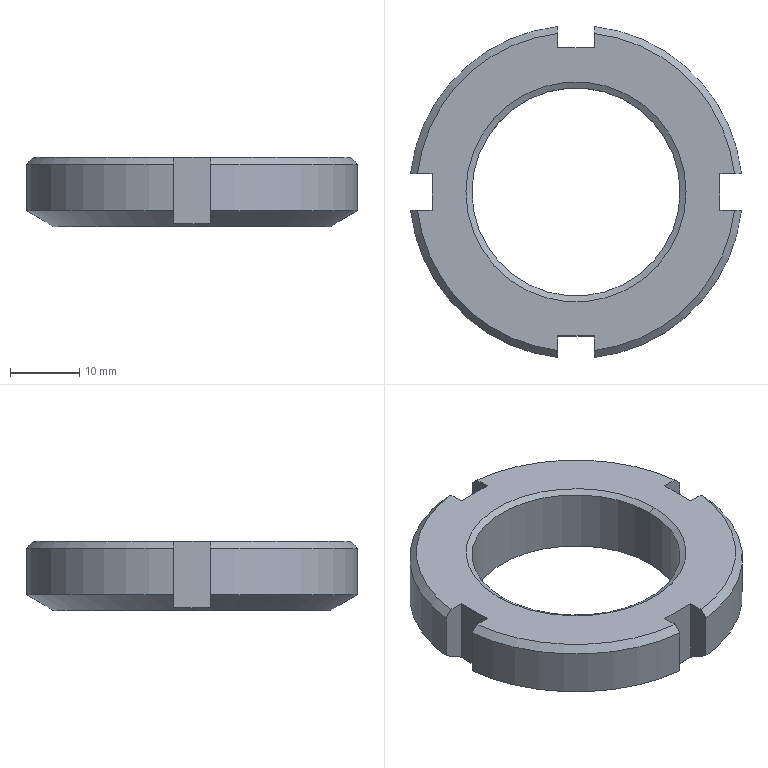Part | SolidWorks | features Chamfer 3, CirPattern 1, Cut 1, Extrusion 1 | 1 solid | 30 faces | box 47.706 x 47.706 x 10 mm | volume 9680 mm3 | plane 14 | cone 10 | cylinder 6 | commonest cylinder face diameters 48 x4 30 x2
STEP:
#1=CARTESIAN_POINT('',(-15.,0.,9.5));
#2=VERTEX_POINT('',#1);
#3=CARTESIAN_POINT('',(15.,0.,9.5));
#4=VERTEX_POINT('',#3);
#5=CARTESIAN_POINT('',(0.,0.,9.5));
#6=DIRECTION('',(0.,0.,1.));
#7=DIRECTION('',(1.,0.,0.));
#8=AXIS2_PLACEMENT_3D('',#5,#6,#7);
#9=CIRCLE('',#8,15.);
#10=EDGE_CURVE('',#2,#4,#9,.T.);
#11=ORIENTED_EDGE('',*,*,#10,.F.);
#12=CARTESIAN_POINT('',(-15.866,0.,10.));
#13=VERTEX_POINT('',#12);
#14=CARTESIAN_POINT('',(-15.,0.,9.5));
#15=DIRECTION('',(-0.866,0.,0.5));
#16=VECTOR('',#15,1000.);
#17=LINE('',#14,#16);
#18=EDGE_CURVE('',#2,#13,#17,.T.);
#19=ORIENTED_EDGE('',*,*,#18,.T.);
#20=CARTESIAN_POINT('',(15.866,0.,10.));
#21=VERTEX_POINT('',#20);
#22=CARTESIAN_POINT('',(0.,0.,10.));
#23=DIRECTION('',(0.,0.,-1.));
#24=DIRECTION('',(1.,0.,0.));
#25=AXIS2_PLACEMENT_3D('',#22,#23,#24);
#26=CIRCLE('',#25,15.866);
#27=EDGE_CURVE('',#21,#13,#26,.T.);
#28=ORIENTED_EDGE('',*,*,#27,.F.);
#29=CARTESIAN_POINT('',(15.,0.,9.5));
#30=DIRECTION('',(0.866,0.,0.5));
#31=VECTOR('',#30,1000.);
#32=LINE('',#29,#31);
#33=EDGE_CURVE('',#4,#21,#32,.T.);
#34=ORIENTED_EDGE('',*,*,#33,.F.);
#35=EDGE_LOOP('',(#11,#19,#28,#34));
#36=FACE_OUTER_BOUND('',#35,.T.);
#37=CARTESIAN_POINT('',(0.,0.,9.5));
#38=DIRECTION('',(0.,0.,1.));
#39=DIRECTION('',(1.,0.,0.));
#40=AXIS2_PLACEMENT_3D('',#37,#38,#39);
#41=CONICAL_SURFACE('',#40,15.,1.047);
#42=ADVANCED_FACE('',(#36),#41,.F.);
#43=CARTESIAN_POINT('',(15.,0.,0.5));
#44=VERTEX_POINT('',#43);
#45=CARTESIAN_POINT('',(-15.,0.,0.5));
#46=VERTEX_POINT('',#45);
#47=CARTESIAN_POINT('',(0.,0.,0.5));
#48=DIRECTION('',(0.,0.,-1.));
#49=DIRECTION('',(1.,0.,0.));
#50=AXIS2_PLACEMENT_3D('',#47,#48,#49);
#51=CIRCLE('',#50,15.);
#52=EDGE_CURVE('',#44,#46,#51,.T.);
#53=ORIENTED_EDGE('',*,*,#52,.F.);
#54=CARTESIAN_POINT('',(15.866,0.,0.));
#55=VERTEX_POINT('',#54);
#56=CARTESIAN_POINT('',(15.866,0.,0.));
#57=DIRECTION('',(0.866,0.,-0.5));
#58=VECTOR('',#57,1000.);
#59=LINE('',#56,#58);
#60=EDGE_CURVE('',#44,#55,#59,.T.);
#61=ORIENTED_EDGE('',*,*,#60,.T.);
#62=CARTESIAN_POINT('',(-15.866,0.,0.));
#63=VERTEX_POINT('',#62);
#64=CARTESIAN_POINT('',(0.,0.,0.));
#65=DIRECTION('',(0.,0.,1.));
#66=DIRECTION('',(1.,0.,0.));
#67=AXIS2_PLACEMENT_3D('',#64,#65,#66);
#68=CIRCLE('',#67,15.866);
#69=EDGE_CURVE('',#63,#55,#68,.T.);
#70=ORIENTED_EDGE('',*,*,#69,.F.);
#71=CARTESIAN_POINT('',(-15.866,0.,0.));
#72=DIRECTION('',(-0.866,0.,-0.5));
#73=VECTOR('',#72,1000.);
#74=LINE('',#71,#73);
#75=EDGE_CURVE('',#46,#63,#74,.T.);
#76=ORIENTED_EDGE('',*,*,#75,.F.);
#77=EDGE_LOOP('',(#53,#61,#70,#76));
#78=FACE_OUTER_BOUND('',#77,.T.);
#79=CARTESIAN_POINT('',(0.,0.,0.));
#80=DIRECTION('',(0.,0.,-1.));
#81=DIRECTION('',(-1.,0.,0.));
#82=AXIS2_PLACEMENT_3D('',#79,#80,#81);
#83=CONICAL_SURFACE('',#82,15.866,1.047);
#84=ADVANCED_FACE('',(#78),#83,.F.);
#85=CARTESIAN_POINT('',(-20.,0.,0.));
#86=VERTEX_POINT('',#85);
#87=CARTESIAN_POINT('',(20.,0.,0.));
#88=VERTEX_POINT('',#87);
#89=CARTESIAN_POINT('',(0.,0.,0.));
#90=DIRECTION('',(0.,0.,-1.));
#91=DIRECTION('',(1.,0.,0.));
#92=AXIS2_PLACEMENT_3D('',#89,#90,#91);
#93=CIRCLE('',#92,20.);
#94=EDGE_CURVE('',#86,#88,#93,.T.);
#95=ORIENTED_EDGE('',*,*,#94,.F.);
#96=CARTESIAN_POINT('',(-20.753,0.,0.4349));
#97=VERTEX_POINT('',#96);
#98=CARTESIAN_POINT('',(-24.,0.,2.309));
#99=DIRECTION('',(-0.866,0.,0.5));
#100=VECTOR('',#99,1000.);
#101=LINE('',#98,#100);
#102=EDGE_CURVE('',#86,#97,#101,.T.);
#103=ORIENTED_EDGE('',*,*,#102,.T.);
#104=CARTESIAN_POINT('',(-20.753,2.65,0.5322));
#105=VERTEX_POINT('',#104);
#106=CARTESIAN_POINT('',(-20.753,2.65,0.5322));
#107=CARTESIAN_POINT('',(-20.753,1.77,0.4678));
#108=CARTESIAN_POINT('',(-20.753,0.8866,0.4349));
#109=CARTESIAN_POINT('',(-20.753,0.,0.4349));
#110=B_SPLINE_CURVE_WITH_KNOTS('',3,(#106,#107,#108,#109),.UNSPECIFIED.,.F.,.F.,(4,4),(0.007091,0.009737),.UNSPECIFIED.);
#111=EDGE_CURVE('',#105,#97,#110,.T.);
#112=ORIENTED_EDGE('',*,*,#111,.F.);
#113=CARTESIAN_POINT('',(-23.853,2.65,2.309));
#114=VERTEX_POINT('',#113);
#115=CARTESIAN_POINT('',(-23.853,2.65,2.309));
#116=CARTESIAN_POINT('',(-22.82,2.65,1.717));
#117=CARTESIAN_POINT('',(-21.787,2.65,1.124));
#118=CARTESIAN_POINT('',(-20.753,2.65,0.5322));
#119=B_SPLINE_CURVE_WITH_KNOTS('',3,(#115,#116,#117,#118),.UNSPECIFIED.,.F.,.F.,(4,4),(0.00673,0.0103),.UNSPECIFIED.);
#120=EDGE_CURVE('',#114,#105,#119,.T.);
#121=ORIENTED_EDGE('',*,*,#120,.F.);
#122=CARTESIAN_POINT('',(-2.65,23.853,2.309));
#123=VERTEX_POINT('',#122);
#124=CARTESIAN_POINT('',(0.,0.,2.309));
#125=DIRECTION('',(0.,0.,1.));
#126=DIRECTION('',(1.,0.,0.));
#127=AXIS2_PLACEMENT_3D('',#124,#125,#126);
#128=CIRCLE('',#127,24.);
#129=EDGE_CURVE('',#123,#114,#128,.T.);
#130=ORIENTED_EDGE('',*,*,#129,.F.);
#131=CARTESIAN_POINT('',(-2.65,20.753,0.5322));
#132=VERTEX_POINT('',#131);
#133=CARTESIAN_POINT('',(-2.65,20.753,0.5322));
#134=CARTESIAN_POINT('',(-2.65,21.787,1.124));
#135=CARTESIAN_POINT('',(-2.65,22.82,1.717));
#136=CARTESIAN_POINT('',(-2.65,23.853,2.309));
#137=B_SPLINE_CURVE_WITH_KNOTS('',3,(#133,#134,#135,#136),.UNSPECIFIED.,.F.,.F.,(4,4),(0.006995,0.01057),.UNSPECIFIED.);
#138=EDGE_CURVE('',#132,#123,#137,.T.);
#139=ORIENTED_EDGE('',*,*,#138,.F.);
#140=CARTESIAN_POINT('',(2.65,20.753,0.5322));
#141=VERTEX_POINT('',#140);
#142=CARTESIAN_POINT('',(2.65,20.753,0.5322));
#143=CARTESIAN_POINT('',(1.773,20.753,0.468));
#144=CARTESIAN_POINT('',(0.8926,20.753,0.4351));
#145=CARTESIAN_POINT('',(-0.8746,20.753,0.4347));
#146=CARTESIAN_POINT('',(-1.764,20.753,0.4674));
#147=CARTESIAN_POINT('',(-2.65,20.753,0.5322));
#148=B_SPLINE_CURVE_WITH_KNOTS('',3,(#142,#143,#144,#145,#146,#147),.UNSPECIFIED.,.F.,.F.,(4,2,4),(0.007091,0.009729,0.01237),.UNSPECIFIED.);
#149=EDGE_CURVE('',#141,#132,#148,.T.);
#150=ORIENTED_EDGE('',*,*,#149,.F.);
#151=CARTESIAN_POINT('',(2.65,23.853,2.309));
#152=VERTEX_POINT('',#151);
#153=CARTESIAN_POINT('',(2.65,23.853,2.309));
#154=CARTESIAN_POINT('',(2.65,22.82,1.717));
#155=CARTESIAN_POINT('',(2.65,21.787,1.124));
#156=CARTESIAN_POINT('',(2.65,20.753,0.5322));
#157=B_SPLINE_CURVE_WITH_KNOTS('',3,(#153,#154,#155,#156),.UNSPECIFIED.,.F.,.F.,(4,4),(0.004139,0.007712),.UNSPECIFIED.);
#158=EDGE_CURVE('',#152,#141,#157,.T.);
#159=ORIENTED_EDGE('',*,*,#158,.F.);
#160=CARTESIAN_POINT('',(23.853,2.65,2.309));
#161=VERTEX_POINT('',#160);
#162=CARTESIAN_POINT('',(0.,0.,2.309));
#163=DIRECTION('',(0.,0.,1.));
#164=DIRECTION('',(1.,0.,0.));
#165=AXIS2_PLACEMENT_3D('',#162,#163,#164);
#166=CIRCLE('',#165,24.);
#167=EDGE_CURVE('',#161,#152,#166,.T.);
#168=ORIENTED_EDGE('',*,*,#167,.F.);
#169=CARTESIAN_POINT('',(20.753,2.65,0.5322));
#170=VERTEX_POINT('',#169);
#171=CARTESIAN_POINT('',(20.753,2.65,0.5322));
#172=CARTESIAN_POINT('',(21.787,2.65,1.124));
#173=CARTESIAN_POINT('',(22.82,2.65,1.717));
#174=CARTESIAN_POINT('',(23.853,2.65,2.309));
#175=B_SPLINE_CURVE_WITH_KNOTS('',3,(#171,#172,#173,#174),.UNSPECIFIED.,.F.,.F.,(4,4),(0.006995,0.01057),.UNSPECIFIED.);
#176=EDGE_CURVE('',#170,#161,#175,.T.);
#177=ORIENTED_EDGE('',*,*,#176,.F.);
#178=CARTESIAN_POINT('',(20.753,0.,0.4349));
#179=VERTEX_POINT('',#178);
#180=CARTESIAN_POINT('',(20.753,0.,0.4349));
#181=CARTESIAN_POINT('',(20.753,0.8866,0.4349));
#182=CARTESIAN_POINT('',(20.753,1.77,0.4678));
#183=CARTESIAN_POINT('',(20.753,2.65,0.5322));
#184=B_SPLINE_CURVE_WITH_KNOTS('',3,(#180,#181,#182,#183),.UNSPECIFIED.,.F.,.F.,(4,4),(0.01366,0.01632),.UNSPECIFIED.);
#185=EDGE_CURVE('',#179,#170,#184,.T.);
#186=ORIENTED_EDGE('',*,*,#185,.F.);
#187=CARTESIAN_POINT('',(24.,0.,2.309));
#188=DIRECTION('',(0.866,0.,0.5));
#189=VECTOR('',#188,1000.);
#190=LINE('',#187,#189);
#191=EDGE_CURVE('',#88,#179,#190,.T.);
#192=ORIENTED_EDGE('',*,*,#191,.F.);
#193=EDGE_LOOP('',(#95,#103,#112,#121,#130,#139,#150,#159,#168,#177,#186,#192));
#194=FACE_OUTER_BOUND('',#193,.T.);
#195=CARTESIAN_POINT('',(0.,0.,2.309));
#196=DIRECTION('',(0.,0.,1.));
#197=DIRECTION('',(1.,0.,0.));
#198=AXIS2_PLACEMENT_3D('',#195,#196,#197);
#199=CONICAL_SURFACE('',#198,24.,1.047);
#200=ADVANCED_FACE('',(#194),#199,.T.);
#201=ORIENTED_EDGE('',*,*,#10,.T.);
#202=CARTESIAN_POINT('',(15.,0.,10.));
#203=DIRECTION('',(0.,0.,-1.));
#204=VECTOR('',#203,1000.);
#205=LINE('',#202,#204);
#206=EDGE_CURVE('',#4,#44,#205,.T.);
#207=ORIENTED_EDGE('',*,*,#206,.T.);
#208=ORIENTED_EDGE('',*,*,#52,.T.);
#209=CARTESIAN_POINT('',(-15.,0.,10.));
#210=DIRECTION('',(0.,0.,-1.));
#211=VECTOR('',#210,1000.);
#212=LINE('',#209,#211);
#213=EDGE_CURVE('',#2,#46,#212,.T.);
#214=ORIENTED_EDGE('',*,*,#213,.F.);
#215=EDGE_LOOP('',(#201,#207,#208,#214));
#216=FACE_OUTER_BOUND('',#215,.T.);
#217=CARTESIAN_POINT('',(0.,0.,10.));
#218=DIRECTION('',(0.,0.,-1.));
#219=DIRECTION('',(-1.,0.,0.));
#220=AXIS2_PLACEMENT_3D('',#217,#218,#219);
#221=CYLINDRICAL_SURFACE('',#220,15.);
#222=ADVANCED_FACE('',(#216),#221,.F.);
#223=CARTESIAN_POINT('',(2.65,23.853,9.));
#224=VERTEX_POINT('',#223);
#225=CARTESIAN_POINT('',(23.853,2.65,9.));
#226=VERTEX_POINT('',#225);
#227=CARTESIAN_POINT('',(0.,0.,9.));
#228=DIRECTION('',(0.,0.,-1.));
#229=DIRECTION('',(1.,0.,0.));
#230=AXIS2_PLACEMENT_3D('',#227,#228,#229);
#231=CIRCLE('',#230,24.);
#232=EDGE_CURVE('',#224,#226,#231,.T.);
#233=ORIENTED_EDGE('',*,*,#232,.T.);
#234=CARTESIAN_POINT('',(23.853,2.65,0.));
#235=DIRECTION('',(0.,0.,1.));
#236=VECTOR('',#235,1000.);
#237=LINE('',#234,#236);
#238=EDGE_CURVE('',#161,#226,#237,.T.);
#239=ORIENTED_EDGE('',*,*,#238,.F.);
#240=ORIENTED_EDGE('',*,*,#167,.T.);
#241=CARTESIAN_POINT('',(2.65,23.853,0.));
#242=DIRECTION('',(0.,0.,1.));
#243=VECTOR('',#242,1000.);
#244=LINE('',#241,#243);
#245=EDGE_CURVE('',#152,#224,#244,.T.);
#246=ORIENTED_EDGE('',*,*,#245,.T.);
#247=EDGE_LOOP('',(#233,#239,#240,#246));
#248=FACE_OUTER_BOUND('',#247,.T.);
#249=CARTESIAN_POINT('',(0.,0.,10.));
#250=DIRECTION('',(0.,0.,-1.));
#251=DIRECTION('',(-1.,0.,0.));
#252=AXIS2_PLACEMENT_3D('',#249,#250,#251);
#253=CYLINDRICAL_SURFACE('',#252,24.);
#254=ADVANCED_FACE('',(#248),#253,.T.);
#255=CARTESIAN_POINT('',(22.847,2.65,10.));
#256=VERTEX_POINT('',#255);
#257=CARTESIAN_POINT('',(23.853,2.65,9.));
#258=CARTESIAN_POINT('',(23.575,2.65,9.277));
#259=CARTESIAN_POINT('',(23.297,2.65,9.553));
#260=CARTESIAN_POINT('',(23.018,2.65,9.83));
#261=CARTESIAN_POINT('',(22.961,2.65,9.886));
#262=CARTESIAN_POINT('',(22.904,2.65,9.943));
#263=CARTESIAN_POINT('',(22.847,2.65,10.));
#264=B_SPLINE_CURVE_WITH_KNOTS('',3,(#257,#258,#259,#260,#261,#262,#263),.UNSPECIFIED.,.F.,.F.,(4,3,4),(0.005158,0.006335,0.006577),.UNSPECIFIED.);
#265=EDGE_CURVE('',#226,#256,#264,.T.);
#266=ORIENTED_EDGE('',*,*,#265,.F.);
#267=ORIENTED_EDGE('',*,*,#232,.F.);
#268=CARTESIAN_POINT('',(2.65,22.847,10.));
#269=VERTEX_POINT('',#268);
#270=CARTESIAN_POINT('',(2.65,22.847,10.));
#271=CARTESIAN_POINT('',(2.65,22.904,9.943));
#272=CARTESIAN_POINT('',(2.65,22.961,9.886));
#273=CARTESIAN_POINT('',(2.65,23.018,9.83));
#274=CARTESIAN_POINT('',(2.65,23.297,9.553));
#275=CARTESIAN_POINT('',(2.65,23.575,9.277));
#276=CARTESIAN_POINT('',(2.65,23.853,9.));
#277=B_SPLINE_CURVE_WITH_KNOTS('',3,(#270,#271,#272,#273,#274,#275,#276),.UNSPECIFIED.,.F.,.F.,(4,3,4),(0.006094,0.006335,0.007512),.UNSPECIFIED.);
#278=EDGE_CURVE('',#269,#224,#277,.T.);
#279=ORIENTED_EDGE('',*,*,#278,.F.);
#280=CARTESIAN_POINT('',(0.,0.,10.));
#281=DIRECTION('',(0.,0.,1.));
#282=DIRECTION('',(1.,0.,0.));
#283=AXIS2_PLACEMENT_3D('',#280,#281,#282);
#284=CIRCLE('',#283,23.);
#285=EDGE_CURVE('',#256,#269,#284,.T.);
#286=ORIENTED_EDGE('',*,*,#285,.F.);
#287=EDGE_LOOP('',(#266,#267,#279,#286));
#288=FACE_OUTER_BOUND('',#287,.T.);
#289=CARTESIAN_POINT('',(0.,0.,10.));
#290=DIRECTION('',(0.,0.,-1.));
#291=DIRECTION('',(-1.,0.,0.));
#292=AXIS2_PLACEMENT_3D('',#289,#290,#291);
#293=CONICAL_SURFACE('',#292,23.,0.7854);
#294=ADVANCED_FACE('',(#288),#293,.T.);
#295=CARTESIAN_POINT('',(-23.853,2.65,9.));
#296=VERTEX_POINT('',#295);
#297=CARTESIAN_POINT('',(-2.65,23.853,9.));
#298=VERTEX_POINT('',#297);
#299=CARTESIAN_POINT('',(0.,0.,9.));
#300=DIRECTION('',(0.,0.,-1.));
#301=DIRECTION('',(1.,0.,0.));
#302=AXIS2_PLACEMENT_3D('',#299,#300,#301);
#303=CIRCLE('',#302,24.);
#304=EDGE_CURVE('',#296,#298,#303,.T.);
#305=ORIENTED_EDGE('',*,*,#304,.T.);
#306=CARTESIAN_POINT('',(-2.65,23.853,0.));
#307=DIRECTION('',(0.,0.,1.));
#308=VECTOR('',#307,1000.);
#309=LINE('',#306,#308);
#310=EDGE_CURVE('',#123,#298,#309,.T.);
#311=ORIENTED_EDGE('',*,*,#310,.F.);
#312=ORIENTED_EDGE('',*,*,#129,.T.);
#313=CARTESIAN_POINT('',(-23.853,2.65,0.));
#314=DIRECTION('',(0.,0.,1.));
#315=VECTOR('',#314,1000.);
#316=LINE('',#313,#315);
#317=EDGE_CURVE('',#114,#296,#316,.T.);
#318=ORIENTED_EDGE('',*,*,#317,.T.);
#319=EDGE_LOOP('',(#305,#311,#312,#318));
#320=FACE_OUTER_BOUND('',#319,.T.);
#321=CARTESIAN_POINT('',(0.,0.,10.));
#322=DIRECTION('',(0.,0.,-1.));
#323=DIRECTION('',(-1.,0.,0.));
#324=AXIS2_PLACEMENT_3D('',#321,#322,#323);
#325=CYLINDRICAL_SURFACE('',#324,24.);
#326=ADVANCED_FACE('',(#320),#325,.T.);
#327=CARTESIAN_POINT('',(-2.65,22.847,10.));
#328=VERTEX_POINT('',#327);
#329=CARTESIAN_POINT('',(-2.65,23.853,9.));
#330=CARTESIAN_POINT('',(-2.65,23.575,9.277));
#331=CARTESIAN_POINT('',(-2.65,23.297,9.553));
#332=CARTESIAN_POINT('',(-2.65,23.018,9.83));
#333=CARTESIAN_POINT('',(-2.65,22.961,9.886));
#334=CARTESIAN_POINT('',(-2.65,22.904,9.943));
#335=CARTESIAN_POINT('',(-2.65,22.847,10.));
#336=B_SPLINE_CURVE_WITH_KNOTS('',3,(#329,#330,#331,#332,#333,#334,#335),.UNSPECIFIED.,.F.,.F.,(4,3,4),(0.005158,0.006335,0.006577),.UNSPECIFIED.);
#337=EDGE_CURVE('',#298,#328,#336,.T.);
#338=ORIENTED_EDGE('',*,*,#337,.F.);
#339=ORIENTED_EDGE('',*,*,#304,.F.);
#340=CARTESIAN_POINT('',(-22.847,2.65,10.));
#341=VERTEX_POINT('',#340);
#342=CARTESIAN_POINT('',(-22.847,2.65,10.));
#343=CARTESIAN_POINT('',(-23.034,2.65,9.814));
#344=CARTESIAN_POINT('',(-23.221,2.65,9.628));
#345=CARTESIAN_POINT('',(-23.408,2.65,9.442));
#346=CARTESIAN_POINT('',(-23.557,2.65,9.295));
#347=CARTESIAN_POINT('',(-23.705,2.65,9.147));
#348=CARTESIAN_POINT('',(-23.853,2.65,9.));
#349=B_SPLINE_CURVE_WITH_KNOTS('',3,(#342,#343,#344,#345,#346,#347,#348),.UNSPECIFIED.,.F.,.F.,(4,3,4),(0.005544,0.006335,0.006963),.UNSPECIFIED.);
#350=EDGE_CURVE('',#341,#296,#349,.T.);
#351=ORIENTED_EDGE('',*,*,#350,.F.);
#352=CARTESIAN_POINT('',(0.,0.,10.));
#353=DIRECTION('',(0.,0.,1.));
#354=DIRECTION('',(1.,0.,0.));
#355=AXIS2_PLACEMENT_3D('',#352,#353,#354);
#356=CIRCLE('',#355,23.);
#357=EDGE_CURVE('',#328,#341,#356,.T.);
#358=ORIENTED_EDGE('',*,*,#357,.F.);
#359=EDGE_LOOP('',(#338,#339,#351,#358));
#360=FACE_OUTER_BOUND('',#359,.T.);
#361=CARTESIAN_POINT('',(0.,0.,10.));
#362=DIRECTION('',(0.,0.,-1.));
#363=DIRECTION('',(-1.,0.,0.));
#364=AXIS2_PLACEMENT_3D('',#361,#362,#363);
#365=CONICAL_SURFACE('',#364,23.,0.7854);
#366=ADVANCED_FACE('',(#360),#365,.T.);
#367=CARTESIAN_POINT('',(-2.65,-23.853,9.));
#368=VERTEX_POINT('',#367);
#369=CARTESIAN_POINT('',(-23.853,-2.65,9.));
#370=VERTEX_POINT('',#369);
#371=CARTESIAN_POINT('',(0.,0.,9.));
#372=DIRECTION('',(0.,0.,-1.));
#373=DIRECTION('',(1.,0.,0.));
#374=AXIS2_PLACEMENT_3D('',#371,#372,#373);
#375=CIRCLE('',#374,24.);
#376=EDGE_CURVE('',#368,#370,#375,.T.);
#377=ORIENTED_EDGE('',*,*,#376,.T.);
#378=CARTESIAN_POINT('',(-23.853,-2.65,2.309));
#379=VERTEX_POINT('',#378);
#380=CARTESIAN_POINT('',(-23.853,-2.65,0.));
#381=DIRECTION('',(0.,0.,1.));
#382=VECTOR('',#381,1000.);
#383=LINE('',#380,#382);
#384=EDGE_CURVE('',#379,#370,#383,.T.);
#385=ORIENTED_EDGE('',*,*,#384,.F.);
#386=CARTESIAN_POINT('',(-2.65,-23.853,2.309));
#387=VERTEX_POINT('',#386);
#388=CARTESIAN_POINT('',(0.,0.,2.309));
#389=DIRECTION('',(0.,0.,1.));
#390=DIRECTION('',(1.,0.,0.));
#391=AXIS2_PLACEMENT_3D('',#388,#389,#390);
#392=CIRCLE('',#391,24.);
#393=EDGE_CURVE('',#379,#387,#392,.T.);
#394=ORIENTED_EDGE('',*,*,#393,.T.);
#395=CARTESIAN_POINT('',(-2.65,-23.853,0.));
#396=DIRECTION('',(0.,0.,1.));
#397=VECTOR('',#396,1000.);
#398=LINE('',#395,#397);
#399=EDGE_CURVE('',#387,#368,#398,.T.);
#400=ORIENTED_EDGE('',*,*,#399,.T.);
#401=EDGE_LOOP('',(#377,#385,#394,#400));
#402=FACE_OUTER_BOUND('',#401,.T.);
#403=CARTESIAN_POINT('',(0.,0.,10.));
#404=DIRECTION('',(0.,0.,-1.));
#405=DIRECTION('',(-1.,0.,0.));
#406=AXIS2_PLACEMENT_3D('',#403,#404,#405);
#407=CYLINDRICAL_SURFACE('',#406,24.);
#408=ADVANCED_FACE('',(#402),#407,.T.);
#409=CARTESIAN_POINT('',(-22.847,-2.65,10.));
#410=VERTEX_POINT('',#409);
#411=CARTESIAN_POINT('',(-23.853,-2.65,9.));
#412=CARTESIAN_POINT('',(-23.705,-2.65,9.147));
#413=CARTESIAN_POINT('',(-23.557,-2.65,9.295));
#414=CARTESIAN_POINT('',(-23.408,-2.65,9.442));
#415=CARTESIAN_POINT('',(-23.221,-2.65,9.628));
#416=CARTESIAN_POINT('',(-23.034,-2.65,9.814));
#417=CARTESIAN_POINT('',(-22.847,-2.65,10.));
#418=B_SPLINE_CURVE_WITH_KNOTS('',3,(#411,#412,#413,#414,#415,#416,#417),.UNSPECIFIED.,.F.,.F.,(4,3,4),(0.005708,0.006335,0.007127),.UNSPECIFIED.);
#419=EDGE_CURVE('',#370,#410,#418,.T.);
#420=ORIENTED_EDGE('',*,*,#419,.F.);
#421=ORIENTED_EDGE('',*,*,#376,.F.);
#422=CARTESIAN_POINT('',(-2.65,-22.847,10.));
#423=VERTEX_POINT('',#422);
#424=CARTESIAN_POINT('',(-2.65,-22.847,10.));
#425=CARTESIAN_POINT('',(-2.65,-23.034,9.814));
#426=CARTESIAN_POINT('',(-2.65,-23.221,9.628));
#427=CARTESIAN_POINT('',(-2.65,-23.408,9.442));
#428=CARTESIAN_POINT('',(-2.65,-23.557,9.295));
#429=CARTESIAN_POINT('',(-2.65,-23.705,9.147));
#430=CARTESIAN_POINT('',(-2.65,-23.853,9.));
#431=B_SPLINE_CURVE_WITH_KNOTS('',3,(#424,#425,#426,#427,#428,#429,#430),.UNSPECIFIED.,.F.,.F.,(4,3,4),(0.005544,0.006335,0.006963),.UNSPECIFIED.);
#432=EDGE_CURVE('',#423,#368,#431,.T.);
#433=ORIENTED_EDGE('',*,*,#432,.F.);
#434=CARTESIAN_POINT('',(0.,0.,10.));
#435=DIRECTION('',(0.,0.,1.));
#436=DIRECTION('',(1.,0.,0.));
#437=AXIS2_PLACEMENT_3D('',#434,#435,#436);
#438=CIRCLE('',#437,23.);
#439=EDGE_CURVE('',#410,#423,#438,.T.);
#440=ORIENTED_EDGE('',*,*,#439,.F.);
#441=EDGE_LOOP('',(#420,#421,#433,#440));
#442=FACE_OUTER_BOUND('',#441,.T.);
#443=CARTESIAN_POINT('',(0.,0.,10.));
#444=DIRECTION('',(0.,0.,-1.));
#445=DIRECTION('',(-1.,0.,0.));
#446=AXIS2_PLACEMENT_3D('',#443,#444,#445);
#447=CONICAL_SURFACE('',#446,23.,0.7854);
#448=ADVANCED_FACE('',(#442),#447,.T.);
#449=ORIENTED_EDGE('',*,*,#27,.T.);
#450=CARTESIAN_POINT('',(0.,0.,10.));
#451=DIRECTION('',(0.,0.,-1.));
#452=DIRECTION('',(1.,0.,0.));
#453=AXIS2_PLACEMENT_3D('',#450,#451,#452);
#454=CIRCLE('',#453,15.866);
#455=EDGE_CURVE('',#13,#21,#454,.T.);
#456=ORIENTED_EDGE('',*,*,#455,.T.);
#457=EDGE_LOOP('',(#449,#456));
#458=FACE_BOUND('',#457,.T.);
#459=CARTESIAN_POINT('',(20.753,2.65,10.));
#460=VERTEX_POINT('',#459);
#461=CARTESIAN_POINT('',(20.753,2.65,10.));
#462=DIRECTION('',(-1.,0.,0.));
#463=VECTOR('',#462,1000.);
#464=LINE('',#461,#463);
#465=EDGE_CURVE('',#256,#460,#464,.T.);
#466=ORIENTED_EDGE('',*,*,#465,.F.);
#467=ORIENTED_EDGE('',*,*,#285,.T.);
#468=CARTESIAN_POINT('',(2.65,20.753,10.));
#469=VERTEX_POINT('',#468);
#470=CARTESIAN_POINT('',(2.65,20.753,10.));
#471=DIRECTION('',(0.,1.,0.));
#472=VECTOR('',#471,1000.);
#473=LINE('',#470,#472);
#474=EDGE_CURVE('',#469,#269,#473,.T.);
#475=ORIENTED_EDGE('',*,*,#474,.F.);
#476=CARTESIAN_POINT('',(-2.65,20.753,10.));
#477=VERTEX_POINT('',#476);
#478=CARTESIAN_POINT('',(2.65,20.753,10.));
#479=DIRECTION('',(1.,0.,0.));
#480=VECTOR('',#479,1000.);
#481=LINE('',#478,#480);
#482=EDGE_CURVE('',#477,#469,#481,.T.);
#483=ORIENTED_EDGE('',*,*,#482,.F.);
#484=CARTESIAN_POINT('',(-2.65,20.753,10.));
#485=DIRECTION('',(0.,-1.,0.));
#486=VECTOR('',#485,1000.);
#487=LINE('',#484,#486);
#488=EDGE_CURVE('',#328,#477,#487,.T.);
#489=ORIENTED_EDGE('',*,*,#488,.F.);
#490=ORIENTED_EDGE('',*,*,#357,.T.);
#491=CARTESIAN_POINT('',(-20.753,2.65,10.));
#492=VERTEX_POINT('',#491);
#493=CARTESIAN_POINT('',(-20.753,2.65,10.));
#494=DIRECTION('',(-1.,0.,0.));
#495=VECTOR('',#494,1000.);
#496=LINE('',#493,#495);
#497=EDGE_CURVE('',#492,#341,#496,.T.);
#498=ORIENTED_EDGE('',*,*,#497,.F.);
#499=CARTESIAN_POINT('',(-20.753,-2.65,10.));
#500=VERTEX_POINT('',#499);
#501=CARTESIAN_POINT('',(-20.753,2.65,10.));
#502=DIRECTION('',(0.,1.,0.));
#503=VECTOR('',#502,1000.);
#504=LINE('',#501,#503);
#505=EDGE_CURVE('',#500,#492,#504,.T.);
#506=ORIENTED_EDGE('',*,*,#505,.F.);
#507=CARTESIAN_POINT('',(-20.753,-2.65,10.));
#508=DIRECTION('',(1.,0.,0.));
#509=VECTOR('',#508,1000.);
#510=LINE('',#507,#509);
#511=EDGE_CURVE('',#410,#500,#510,.T.);
#512=ORIENTED_EDGE('',*,*,#511,.F.);
#513=ORIENTED_EDGE('',*,*,#439,.T.);
#514=CARTESIAN_POINT('',(-2.65,-20.753,10.));
#515=VERTEX_POINT('',#514);
#516=CARTESIAN_POINT('',(-2.65,-20.753,10.));
#517=DIRECTION('',(0.,-1.,0.));
#518=VECTOR('',#517,1000.);
#519=LINE('',#516,#518);
#520=EDGE_CURVE('',#515,#423,#519,.T.);
#521=ORIENTED_EDGE('',*,*,#520,.F.);
#522=CARTESIAN_POINT('',(2.65,-20.753,10.));
#523=VERTEX_POINT('',#522);
#524=CARTESIAN_POINT('',(-2.65,-20.753,10.));
#525=DIRECTION('',(-1.,0.,0.));
#526=VECTOR('',#525,1000.);
#527=LINE('',#524,#526);
#528=EDGE_CURVE('',#523,#515,#527,.T.);
#529=ORIENTED_EDGE('',*,*,#528,.F.);
#530=CARTESIAN_POINT('',(2.65,-22.847,10.));
#531=VERTEX_POINT('',#530);
#532=CARTESIAN_POINT('',(2.65,-20.753,10.));
#533=DIRECTION('',(0.,1.,0.));
#534=VECTOR('',#533,1000.);
#535=LINE('',#532,#534);
#536=EDGE_CURVE('',#531,#523,#535,.T.);
#537=ORIENTED_EDGE('',*,*,#536,.F.);
#538=CARTESIAN_POINT('',(22.847,-2.65,10.));
#539=VERTEX_POINT('',#538);
#540=CARTESIAN_POINT('',(0.,0.,10.));
#541=DIRECTION('',(0.,0.,1.));
#542=DIRECTION('',(1.,0.,0.));
#543=AXIS2_PLACEMENT_3D('',#540,#541,#542);
#544=CIRCLE('',#543,23.);
#545=EDGE_CURVE('',#531,#539,#544,.T.);
#546=ORIENTED_EDGE('',*,*,#545,.T.);
#547=CARTESIAN_POINT('',(20.753,-2.65,10.));
#548=VERTEX_POINT('',#547);
#549=CARTESIAN_POINT('',(20.753,-2.65,10.));
#550=DIRECTION('',(1.,0.,0.));
#551=VECTOR('',#550,1000.);
#552=LINE('',#549,#551);
#553=EDGE_CURVE('',#548,#539,#552,.T.);
#554=ORIENTED_EDGE('',*,*,#553,.F.);
#555=CARTESIAN_POINT('',(20.753,-2.65,10.));
#556=DIRECTION('',(0.,-1.,0.));
#557=VECTOR('',#556,1000.);
#558=LINE('',#555,#557);
#559=EDGE_CURVE('',#460,#548,#558,.T.);
#560=ORIENTED_EDGE('',*,*,#559,.F.);
#561=EDGE_LOOP('',(#466,#467,#475,#483,#489,#490,#498,#506,#512,#513,#521,#529,#537,#546,#554,#560));
#562=FACE_OUTER_BOUND('',#561,.T.);
#563=CARTESIAN_POINT('',(0.,0.,10.));
#564=DIRECTION('',(0.,0.,1.));
#565=DIRECTION('',(1.,0.,0.));
#566=AXIS2_PLACEMENT_3D('',#563,#564,#565);
#567=PLANE('',#566);
#568=ADVANCED_FACE('',(#458,#562),#567,.T.);
#569=ORIENTED_EDGE('',*,*,#69,.T.);
#570=CARTESIAN_POINT('',(0.,0.,0.));
#571=DIRECTION('',(0.,0.,1.));
#572=DIRECTION('',(1.,0.,0.));
#573=AXIS2_PLACEMENT_3D('',#570,#571,#572);
#574=CIRCLE('',#573,15.866);
#575=EDGE_CURVE('',#55,#63,#574,.T.);
#576=ORIENTED_EDGE('',*,*,#575,.T.);
#577=EDGE_LOOP('',(#569,#576));
#578=FACE_BOUND('',#577,.T.);
#579=CARTESIAN_POINT('',(0.,0.,0.));
#580=DIRECTION('',(0.,0.,-1.));
#581=DIRECTION('',(1.,0.,0.));
#582=AXIS2_PLACEMENT_3D('',#579,#580,#581);
#583=CIRCLE('',#582,20.);
#584=EDGE_CURVE('',#88,#86,#583,.T.);
#585=ORIENTED_EDGE('',*,*,#584,.T.);
#586=ORIENTED_EDGE('',*,*,#94,.T.);
#587=EDGE_LOOP('',(#585,#586));
#588=FACE_OUTER_BOUND('',#587,.T.);
#589=CARTESIAN_POINT('',(0.,0.,0.));
#590=DIRECTION('',(0.,0.,1.));
#591=DIRECTION('',(1.,0.,0.));
#592=AXIS2_PLACEMENT_3D('',#589,#590,#591);
#593=PLANE('',#592);
#594=ADVANCED_FACE('',(#578,#588),#593,.F.);
#595=CARTESIAN_POINT('',(2.65,-23.853,2.309));
#596=VERTEX_POINT('',#595);
#597=CARTESIAN_POINT('',(23.853,-2.65,2.309));
#598=VERTEX_POINT('',#597);
#599=CARTESIAN_POINT('',(0.,0.,2.309));
#600=DIRECTION('',(0.,0.,1.));
#601=DIRECTION('',(1.,0.,0.));
#602=AXIS2_PLACEMENT_3D('',#599,#600,#601);
#603=CIRCLE('',#602,24.);
#604=EDGE_CURVE('',#596,#598,#603,.T.);
#605=ORIENTED_EDGE('',*,*,#604,.T.);
#606=CARTESIAN_POINT('',(23.853,-2.65,9.));
#607=VERTEX_POINT('',#606);
#608=CARTESIAN_POINT('',(23.853,-2.65,0.));
#609=DIRECTION('',(0.,0.,1.));
#610=VECTOR('',#609,1000.);
#611=LINE('',#608,#610);
#612=EDGE_CURVE('',#598,#607,#611,.T.);
#613=ORIENTED_EDGE('',*,*,#612,.T.);
#614=CARTESIAN_POINT('',(2.65,-23.853,9.));
#615=VERTEX_POINT('',#614);
#616=CARTESIAN_POINT('',(0.,0.,9.));
#617=DIRECTION('',(0.,0.,-1.));
#618=DIRECTION('',(1.,0.,0.));
#619=AXIS2_PLACEMENT_3D('',#616,#617,#618);
#620=CIRCLE('',#619,24.);
#621=EDGE_CURVE('',#607,#615,#620,.T.);
#622=ORIENTED_EDGE('',*,*,#621,.T.);
#623=CARTESIAN_POINT('',(2.65,-23.853,0.));
#624=DIRECTION('',(0.,0.,1.));
#625=VECTOR('',#624,1000.);
#626=LINE('',#623,#625);
#627=EDGE_CURVE('',#596,#615,#626,.T.);
#628=ORIENTED_EDGE('',*,*,#627,.F.);
#629=EDGE_LOOP('',(#605,#613,#622,#628));
#630=FACE_OUTER_BOUND('',#629,.T.);
#631=CARTESIAN_POINT('',(0.,0.,10.));
#632=DIRECTION('',(0.,0.,-1.));
#633=DIRECTION('',(-1.,0.,0.));
#634=AXIS2_PLACEMENT_3D('',#631,#632,#633);
#635=CYLINDRICAL_SURFACE('',#634,24.);
#636=ADVANCED_FACE('',(#630),#635,.T.);
#637=ORIENTED_EDGE('',*,*,#206,.F.);
#638=CARTESIAN_POINT('',(0.,0.,9.5));
#639=DIRECTION('',(0.,0.,1.));
#640=DIRECTION('',(1.,0.,0.));
#641=AXIS2_PLACEMENT_3D('',#638,#639,#640);
#642=CIRCLE('',#641,15.);
#643=EDGE_CURVE('',#4,#2,#642,.T.);
#644=ORIENTED_EDGE('',*,*,#643,.T.);
#645=ORIENTED_EDGE('',*,*,#213,.T.);
#646=CARTESIAN_POINT('',(0.,0.,0.5));
#647=DIRECTION('',(0.,0.,-1.));
#648=DIRECTION('',(1.,0.,0.));
#649=AXIS2_PLACEMENT_3D('',#646,#647,#648);
#650=CIRCLE('',#649,15.);
#651=EDGE_CURVE('',#46,#44,#650,.T.);
#652=ORIENTED_EDGE('',*,*,#651,.T.);
#653=EDGE_LOOP('',(#637,#644,#645,#652));
#654=FACE_OUTER_BOUND('',#653,.T.);
#655=CARTESIAN_POINT('',(0.,0.,10.));
#656=DIRECTION('',(0.,0.,-1.));
#657=DIRECTION('',(-1.,0.,0.));
#658=AXIS2_PLACEMENT_3D('',#655,#656,#657);
#659=CYLINDRICAL_SURFACE('',#658,15.);
#660=ADVANCED_FACE('',(#654),#659,.F.);
#661=CARTESIAN_POINT('',(22.847,-2.65,10.));
#662=CARTESIAN_POINT('',(22.904,-2.65,9.943));
#663=CARTESIAN_POINT('',(22.961,-2.65,9.886));
#664=CARTESIAN_POINT('',(23.018,-2.65,9.83));
#665=CARTESIAN_POINT('',(23.297,-2.65,9.553));
#666=CARTESIAN_POINT('',(23.575,-2.65,9.277));
#667=CARTESIAN_POINT('',(23.853,-2.65,9.));
#668=B_SPLINE_CURVE_WITH_KNOTS('',3,(#661,#662,#663,#664,#665,#666,#667),.UNSPECIFIED.,.F.,.F.,(4,3,4),(0.006094,0.006335,0.007512),.UNSPECIFIED.);
#669=EDGE_CURVE('',#539,#607,#668,.T.);
#670=ORIENTED_EDGE('',*,*,#669,.F.);
#671=ORIENTED_EDGE('',*,*,#545,.F.);
#672=CARTESIAN_POINT('',(2.65,-23.853,9.));
#673=CARTESIAN_POINT('',(2.65,-23.705,9.147));
#674=CARTESIAN_POINT('',(2.65,-23.557,9.295));
#675=CARTESIAN_POINT('',(2.65,-23.408,9.442));
#676=CARTESIAN_POINT('',(2.65,-23.221,9.628));
#677=CARTESIAN_POINT('',(2.65,-23.034,9.814));
#678=CARTESIAN_POINT('',(2.65,-22.847,10.));
#679=B_SPLINE_CURVE_WITH_KNOTS('',3,(#672,#673,#674,#675,#676,#677,#678),.UNSPECIFIED.,.F.,.F.,(4,3,4),(0.005708,0.006335,0.007127),.UNSPECIFIED.);
#680=EDGE_CURVE('',#615,#531,#679,.T.);
#681=ORIENTED_EDGE('',*,*,#680,.F.);
#682=ORIENTED_EDGE('',*,*,#621,.F.);
#683=EDGE_LOOP('',(#670,#671,#681,#682));
#684=FACE_OUTER_BOUND('',#683,.T.);
#685=CARTESIAN_POINT('',(0.,0.,10.));
#686=DIRECTION('',(0.,0.,-1.));
#687=DIRECTION('',(-1.,0.,0.));
#688=AXIS2_PLACEMENT_3D('',#685,#686,#687);
#689=CONICAL_SURFACE('',#688,23.,0.7854);
#690=ADVANCED_FACE('',(#684),#689,.T.);
#691=ORIENTED_EDGE('',*,*,#102,.F.);
#692=ORIENTED_EDGE('',*,*,#584,.F.);
#693=ORIENTED_EDGE('',*,*,#191,.T.);
#694=CARTESIAN_POINT('',(20.753,-2.65,0.5322));
#695=VERTEX_POINT('',#694);
#696=CARTESIAN_POINT('',(20.753,-2.65,0.5322));
#697=CARTESIAN_POINT('',(20.753,-1.767,0.4676));
#698=CARTESIAN_POINT('',(20.753,-0.8806,0.4349));
#699=CARTESIAN_POINT('',(20.753,0.,0.4349));
#700=B_SPLINE_CURVE_WITH_KNOTS('',3,(#696,#697,#698,#699),.UNSPECIFIED.,.F.,.F.,(4,4),(0.01103,0.01366),.UNSPECIFIED.);
#701=EDGE_CURVE('',#695,#179,#700,.T.);
#702=ORIENTED_EDGE('',*,*,#701,.F.);
#703=CARTESIAN_POINT('',(23.853,-2.65,2.309));
#704=CARTESIAN_POINT('',(22.82,-2.65,1.717));
#705=CARTESIAN_POINT('',(21.787,-2.65,1.124));
#706=CARTESIAN_POINT('',(20.753,-2.65,0.5322));
#707=B_SPLINE_CURVE_WITH_KNOTS('',3,(#703,#704,#705,#706),.UNSPECIFIED.,.F.,.F.,(4,4),(0.004139,0.007712),.UNSPECIFIED.);
#708=EDGE_CURVE('',#598,#695,#707,.T.);
#709=ORIENTED_EDGE('',*,*,#708,.F.);
#710=ORIENTED_EDGE('',*,*,#604,.F.);
#711=CARTESIAN_POINT('',(2.65,-20.753,0.5322));
#712=VERTEX_POINT('',#711);
#713=CARTESIAN_POINT('',(2.65,-20.753,0.5322));
#714=CARTESIAN_POINT('',(2.65,-21.787,1.124));
#715=CARTESIAN_POINT('',(2.65,-22.82,1.717));
#716=CARTESIAN_POINT('',(2.65,-23.853,2.309));
#717=B_SPLINE_CURVE_WITH_KNOTS('',3,(#713,#714,#715,#716),.UNSPECIFIED.,.F.,.F.,(4,4),(0.004404,0.007977),.UNSPECIFIED.);
#718=EDGE_CURVE('',#712,#596,#717,.T.);
#719=ORIENTED_EDGE('',*,*,#718,.F.);
#720=CARTESIAN_POINT('',(-2.65,-20.753,0.5322));
#721=VERTEX_POINT('',#720);
#722=CARTESIAN_POINT('',(-2.65,-20.753,0.5322));
#723=CARTESIAN_POINT('',(-1.764,-20.753,0.4674));
#724=CARTESIAN_POINT('',(-0.8746,-20.753,0.4347));
#725=CARTESIAN_POINT('',(0.8926,-20.753,0.4351));
#726=CARTESIAN_POINT('',(1.773,-20.753,0.468));
#727=CARTESIAN_POINT('',(2.65,-20.753,0.5322));
#728=B_SPLINE_CURVE_WITH_KNOTS('',3,(#722,#723,#724,#725,#726,#727),.UNSPECIFIED.,.F.,.F.,(4,2,4),(0.01103,0.01367,0.01632),.UNSPECIFIED.);
#729=EDGE_CURVE('',#721,#712,#728,.T.);
#730=ORIENTED_EDGE('',*,*,#729,.F.);
#731=CARTESIAN_POINT('',(-2.65,-23.853,2.309));
#732=CARTESIAN_POINT('',(-2.65,-22.82,1.717));
#733=CARTESIAN_POINT('',(-2.65,-21.787,1.124));
#734=CARTESIAN_POINT('',(-2.65,-20.753,0.5322));
#735=B_SPLINE_CURVE_WITH_KNOTS('',3,(#731,#732,#733,#734),.UNSPECIFIED.,.F.,.F.,(4,4),(0.00673,0.0103),.UNSPECIFIED.);
#736=EDGE_CURVE('',#387,#721,#735,.T.);
#737=ORIENTED_EDGE('',*,*,#736,.F.);
#738=ORIENTED_EDGE('',*,*,#393,.F.);
#739=CARTESIAN_POINT('',(-20.753,-2.65,0.5322));
#740=VERTEX_POINT('',#739);
#741=CARTESIAN_POINT('',(-20.753,-2.65,0.5322));
#742=CARTESIAN_POINT('',(-21.787,-2.65,1.124));
#743=CARTESIAN_POINT('',(-22.82,-2.65,1.717));
#744=CARTESIAN_POINT('',(-23.853,-2.65,2.309));
#745=B_SPLINE_CURVE_WITH_KNOTS('',3,(#741,#742,#743,#744),.UNSPECIFIED.,.F.,.F.,(4,4),(0.004404,0.007977),.UNSPECIFIED.);
#746=EDGE_CURVE('',#740,#379,#745,.T.);
#747=ORIENTED_EDGE('',*,*,#746,.F.);
#748=CARTESIAN_POINT('',(-20.753,0.,0.4349));
#749=CARTESIAN_POINT('',(-20.753,-0.8806,0.4349));
#750=CARTESIAN_POINT('',(-20.753,-1.767,0.4676));
#751=CARTESIAN_POINT('',(-20.753,-2.65,0.5322));
#752=B_SPLINE_CURVE_WITH_KNOTS('',3,(#748,#749,#750,#751),.UNSPECIFIED.,.F.,.F.,(4,4),(0.009737,0.01237),.UNSPECIFIED.);
#753=EDGE_CURVE('',#97,#740,#752,.T.);
#754=ORIENTED_EDGE('',*,*,#753,.F.);
#755=EDGE_LOOP('',(#691,#692,#693,#702,#709,#710,#719,#730,#737,#738,#747,#754));
#756=FACE_OUTER_BOUND('',#755,.T.);
#757=CARTESIAN_POINT('',(0.,0.,2.309));
#758=DIRECTION('',(0.,0.,1.));
#759=DIRECTION('',(1.,0.,0.));
#760=AXIS2_PLACEMENT_3D('',#757,#758,#759);
#761=CONICAL_SURFACE('',#760,24.,1.047);
#762=ADVANCED_FACE('',(#756),#761,.T.);
#763=ORIENTED_EDGE('',*,*,#729,.T.);
#764=CARTESIAN_POINT('',(2.65,-20.753,0.));
#765=DIRECTION('',(0.,0.,1.));
#766=VECTOR('',#765,1000.);
#767=LINE('',#764,#766);
#768=EDGE_CURVE('',#712,#523,#767,.T.);
#769=ORIENTED_EDGE('',*,*,#768,.T.);
#770=ORIENTED_EDGE('',*,*,#528,.T.);
#771=CARTESIAN_POINT('',(-2.65,-20.753,0.));
#772=DIRECTION('',(0.,0.,1.));
#773=VECTOR('',#772,1000.);
#774=LINE('',#771,#773);
#775=EDGE_CURVE('',#721,#515,#774,.T.);
#776=ORIENTED_EDGE('',*,*,#775,.F.);
#777=EDGE_LOOP('',(#763,#769,#770,#776));
#778=FACE_OUTER_BOUND('',#777,.T.);
#779=CARTESIAN_POINT('',(-2.65,-20.753,0.));
#780=DIRECTION('',(0.,1.,0.));
#781=DIRECTION('',(0.,0.,1.));
#782=AXIS2_PLACEMENT_3D('',#779,#780,#781);
#783=PLANE('',#782);
#784=ADVANCED_FACE('',(#778),#783,.F.);
#785=ORIENTED_EDGE('',*,*,#680,.T.);
#786=ORIENTED_EDGE('',*,*,#536,.T.);
#787=ORIENTED_EDGE('',*,*,#768,.F.);
#788=ORIENTED_EDGE('',*,*,#718,.T.);
#789=ORIENTED_EDGE('',*,*,#627,.T.);
#790=EDGE_LOOP('',(#785,#786,#787,#788,#789));
#791=FACE_OUTER_BOUND('',#790,.T.);
#792=CARTESIAN_POINT('',(2.65,-20.753,0.));
#793=DIRECTION('',(1.,0.,0.));
#794=DIRECTION('',(0.,0.,-1.));
#795=AXIS2_PLACEMENT_3D('',#792,#793,#794);
#796=PLANE('',#795);
#797=ADVANCED_FACE('',(#791),#796,.F.);
#798=ORIENTED_EDGE('',*,*,#432,.T.);
#799=ORIENTED_EDGE('',*,*,#399,.F.);
#800=ORIENTED_EDGE('',*,*,#736,.T.);
#801=ORIENTED_EDGE('',*,*,#775,.T.);
#802=ORIENTED_EDGE('',*,*,#520,.T.);
#803=EDGE_LOOP('',(#798,#799,#800,#801,#802));
#804=FACE_OUTER_BOUND('',#803,.T.);
#805=CARTESIAN_POINT('',(-2.65,-20.753,0.));
#806=DIRECTION('',(-1.,0.,0.));
#807=DIRECTION('',(0.,-1.,0.));
#808=AXIS2_PLACEMENT_3D('',#805,#806,#807);
#809=PLANE('',#808);
#810=ADVANCED_FACE('',(#804),#809,.F.);
#811=ORIENTED_EDGE('',*,*,#111,.T.);
#812=ORIENTED_EDGE('',*,*,#753,.T.);
#813=CARTESIAN_POINT('',(-20.753,-2.65,0.));
#814=DIRECTION('',(0.,0.,1.));
#815=VECTOR('',#814,1000.);
#816=LINE('',#813,#815);
#817=EDGE_CURVE('',#740,#500,#816,.T.);
#818=ORIENTED_EDGE('',*,*,#817,.T.);
#819=ORIENTED_EDGE('',*,*,#505,.T.);
#820=CARTESIAN_POINT('',(-20.753,2.65,0.));
#821=DIRECTION('',(0.,0.,1.));
#822=VECTOR('',#821,1000.);
#823=LINE('',#820,#822);
#824=EDGE_CURVE('',#105,#492,#823,.T.);
#825=ORIENTED_EDGE('',*,*,#824,.F.);
#826=EDGE_LOOP('',(#811,#812,#818,#819,#825));
#827=FACE_OUTER_BOUND('',#826,.T.);
#828=CARTESIAN_POINT('',(-20.753,2.65,0.));
#829=DIRECTION('',(1.,0.,0.));
#830=DIRECTION('',(0.,1.,0.));
#831=AXIS2_PLACEMENT_3D('',#828,#829,#830);
#832=PLANE('',#831);
#833=ADVANCED_FACE('',(#827),#832,.F.);
#834=ORIENTED_EDGE('',*,*,#419,.T.);
#835=ORIENTED_EDGE('',*,*,#511,.T.);
#836=ORIENTED_EDGE('',*,*,#817,.F.);
#837=ORIENTED_EDGE('',*,*,#746,.T.);
#838=ORIENTED_EDGE('',*,*,#384,.T.);
#839=EDGE_LOOP('',(#834,#835,#836,#837,#838));
#840=FACE_OUTER_BOUND('',#839,.T.);
#841=CARTESIAN_POINT('',(-20.753,-2.65,0.));
#842=DIRECTION('',(0.,-1.,0.));
#843=DIRECTION('',(1.,0.,0.));
#844=AXIS2_PLACEMENT_3D('',#841,#842,#843);
#845=PLANE('',#844);
#846=ADVANCED_FACE('',(#840),#845,.F.);
#847=ORIENTED_EDGE('',*,*,#350,.T.);
#848=ORIENTED_EDGE('',*,*,#317,.F.);
#849=ORIENTED_EDGE('',*,*,#120,.T.);
#850=ORIENTED_EDGE('',*,*,#824,.T.);
#851=ORIENTED_EDGE('',*,*,#497,.T.);
#852=EDGE_LOOP('',(#847,#848,#849,#850,#851));
#853=FACE_OUTER_BOUND('',#852,.T.);
#854=CARTESIAN_POINT('',(-20.753,2.65,0.));
#855=DIRECTION('',(0.,1.,0.));
#856=DIRECTION('',(-1.,0.,0.));
#857=AXIS2_PLACEMENT_3D('',#854,#855,#856);
#858=PLANE('',#857);
#859=ADVANCED_FACE('',(#853),#858,.F.);
#860=ORIENTED_EDGE('',*,*,#149,.T.);
#861=CARTESIAN_POINT('',(-2.65,20.753,0.));
#862=DIRECTION('',(0.,0.,1.));
#863=VECTOR('',#862,1000.);
#864=LINE('',#861,#863);
#865=EDGE_CURVE('',#132,#477,#864,.T.);
#866=ORIENTED_EDGE('',*,*,#865,.T.);
#867=ORIENTED_EDGE('',*,*,#482,.T.);
#868=CARTESIAN_POINT('',(2.65,20.753,0.));
#869=DIRECTION('',(0.,0.,1.));
#870=VECTOR('',#869,1000.);
#871=LINE('',#868,#870);
#872=EDGE_CURVE('',#141,#469,#871,.T.);
#873=ORIENTED_EDGE('',*,*,#872,.F.);
#874=EDGE_LOOP('',(#860,#866,#867,#873));
#875=FACE_OUTER_BOUND('',#874,.T.);
#876=CARTESIAN_POINT('',(2.65,20.753,0.));
#877=DIRECTION('',(0.,-1.,0.));
#878=DIRECTION('',(1.,0.,0.));
#879=AXIS2_PLACEMENT_3D('',#876,#877,#878);
#880=PLANE('',#879);
#881=ADVANCED_FACE('',(#875),#880,.F.);
#882=ORIENTED_EDGE('',*,*,#337,.T.);
#883=ORIENTED_EDGE('',*,*,#488,.T.);
#884=ORIENTED_EDGE('',*,*,#865,.F.);
#885=ORIENTED_EDGE('',*,*,#138,.T.);
#886=ORIENTED_EDGE('',*,*,#310,.T.);
#887=EDGE_LOOP('',(#882,#883,#884,#885,#886));
#888=FACE_OUTER_BOUND('',#887,.T.);
#889=CARTESIAN_POINT('',(-2.65,20.753,0.));
#890=DIRECTION('',(-1.,0.,0.));
#891=DIRECTION('',(0.,-1.,0.));
#892=AXIS2_PLACEMENT_3D('',#889,#890,#891);
#893=PLANE('',#892);
#894=ADVANCED_FACE('',(#888),#893,.F.);
#895=ORIENTED_EDGE('',*,*,#278,.T.);
#896=ORIENTED_EDGE('',*,*,#245,.F.);
#897=ORIENTED_EDGE('',*,*,#158,.T.);
#898=ORIENTED_EDGE('',*,*,#872,.T.);
#899=ORIENTED_EDGE('',*,*,#474,.T.);
#900=EDGE_LOOP('',(#895,#896,#897,#898,#899));
#901=FACE_OUTER_BOUND('',#900,.T.);
#902=CARTESIAN_POINT('',(2.65,20.753,0.));
#903=DIRECTION('',(1.,0.,0.));
#904=DIRECTION('',(0.,1.,0.));
#905=AXIS2_PLACEMENT_3D('',#902,#903,#904);
#906=PLANE('',#905);
#907=ADVANCED_FACE('',(#901),#906,.F.);
#908=ORIENTED_EDGE('',*,*,#701,.T.);
#909=ORIENTED_EDGE('',*,*,#185,.T.);
#910=CARTESIAN_POINT('',(20.753,2.65,0.));
#911=DIRECTION('',(0.,0.,1.));
#912=VECTOR('',#911,1000.);
#913=LINE('',#910,#912);
#914=EDGE_CURVE('',#170,#460,#913,.T.);
#915=ORIENTED_EDGE('',*,*,#914,.T.);
#916=ORIENTED_EDGE('',*,*,#559,.T.);
#917=CARTESIAN_POINT('',(20.753,-2.65,0.));
#918=DIRECTION('',(0.,0.,1.));
#919=VECTOR('',#918,1000.);
#920=LINE('',#917,#919);
#921=EDGE_CURVE('',#695,#548,#920,.T.);
#922=ORIENTED_EDGE('',*,*,#921,.F.);
#923=EDGE_LOOP('',(#908,#909,#915,#916,#922));
#924=FACE_OUTER_BOUND('',#923,.T.);
#925=CARTESIAN_POINT('',(20.753,-2.65,0.));
#926=DIRECTION('',(-1.,0.,0.));
#927=DIRECTION('',(0.,-1.,0.));
#928=AXIS2_PLACEMENT_3D('',#925,#926,#927);
#929=PLANE('',#928);
#930=ADVANCED_FACE('',(#924),#929,.F.);
#931=ORIENTED_EDGE('',*,*,#265,.T.);
#932=ORIENTED_EDGE('',*,*,#465,.T.);
#933=ORIENTED_EDGE('',*,*,#914,.F.);
#934=ORIENTED_EDGE('',*,*,#176,.T.);
#935=ORIENTED_EDGE('',*,*,#238,.T.);
#936=EDGE_LOOP('',(#931,#932,#933,#934,#935));
#937=FACE_OUTER_BOUND('',#936,.T.);
#938=CARTESIAN_POINT('',(20.753,2.65,0.));
#939=DIRECTION('',(0.,1.,0.));
#940=DIRECTION('',(-1.,0.,0.));
#941=AXIS2_PLACEMENT_3D('',#938,#939,#940);
#942=PLANE('',#941);
#943=ADVANCED_FACE('',(#937),#942,.F.);
#944=ORIENTED_EDGE('',*,*,#669,.T.);
#945=ORIENTED_EDGE('',*,*,#612,.F.);
#946=ORIENTED_EDGE('',*,*,#708,.T.);
#947=ORIENTED_EDGE('',*,*,#921,.T.);
#948=ORIENTED_EDGE('',*,*,#553,.T.);
#949=EDGE_LOOP('',(#944,#945,#946,#947,#948));
#950=FACE_OUTER_BOUND('',#949,.T.);
#951=CARTESIAN_POINT('',(20.753,-2.65,0.));
#952=DIRECTION('',(0.,-1.,0.));
#953=DIRECTION('',(1.,0.,0.));
#954=AXIS2_PLACEMENT_3D('',#951,#952,#953);
#955=PLANE('',#954);
#956=ADVANCED_FACE('',(#950),#955,.F.);
#957=ORIENTED_EDGE('',*,*,#60,.F.);
#958=ORIENTED_EDGE('',*,*,#651,.F.);
#959=ORIENTED_EDGE('',*,*,#75,.T.);
#960=ORIENTED_EDGE('',*,*,#575,.F.);
#961=EDGE_LOOP('',(#957,#958,#959,#960));
#962=FACE_OUTER_BOUND('',#961,.T.);
#963=CARTESIAN_POINT('',(0.,0.,0.));
#964=DIRECTION('',(0.,0.,-1.));
#965=DIRECTION('',(-1.,0.,0.));
#966=AXIS2_PLACEMENT_3D('',#963,#964,#965);
#967=CONICAL_SURFACE('',#966,15.866,1.047);
#968=ADVANCED_FACE('',(#962),#967,.F.);
#969=ORIENTED_EDGE('',*,*,#18,.F.);
#970=ORIENTED_EDGE('',*,*,#643,.F.);
#971=ORIENTED_EDGE('',*,*,#33,.T.);
#972=ORIENTED_EDGE('',*,*,#455,.F.);
#973=EDGE_LOOP('',(#969,#970,#971,#972));
#974=FACE_OUTER_BOUND('',#973,.T.);
#975=CARTESIAN_POINT('',(0.,0.,9.5));
#976=DIRECTION('',(0.,0.,1.));
#977=DIRECTION('',(1.,0.,0.));
#978=AXIS2_PLACEMENT_3D('',#975,#976,#977);
#979=CONICAL_SURFACE('',#978,15.,1.047);
#980=ADVANCED_FACE('',(#974),#979,.F.);
#981=CLOSED_SHELL('',(#42,#84,#200,#222,#254,#294,#326,#366,#408,#448,#568,#594,#636,#660,#690,#762,#784,#797,#810,#833,#846,#859,#881,#894,#907,#930,#943,#956,#968,#980));
#982=MANIFOLD_SOLID_BREP('',#981);
#983=CARTESIAN_POINT('',(0.,0.,0.));
#984=DIRECTION('',(0.,0.,1.));
#985=DIRECTION('',(1.,0.,0.));
#986=AXIS2_PLACEMENT_3D('',#983,#984,#985);
#987=(LENGTH_UNIT()NAMED_UNIT(*)SI_UNIT(.MILLI.,.METRE.));
#988=UNCERTAINTY_MEASURE_WITH_UNIT(LENGTH_MEASURE(0.00001),#987,'','');
#989=(NAMED_UNIT(*)PLANE_ANGLE_UNIT()SI_UNIT($,.RADIAN.));
#990=(NAMED_UNIT(*)SI_UNIT($,.STERADIAN.)SOLID_ANGLE_UNIT());
#991=(GEOMETRIC_REPRESENTATION_CONTEXT(3)GLOBAL_UNCERTAINTY_ASSIGNED_CONTEXT((#988))GLOBAL_UNIT_ASSIGNED_CONTEXT((#987,#989,#990))REPRESENTATION_CONTEXT('',''));
#992=ADVANCED_BREP_SHAPE_REPRESENTATION('',(#982,#986),#991);